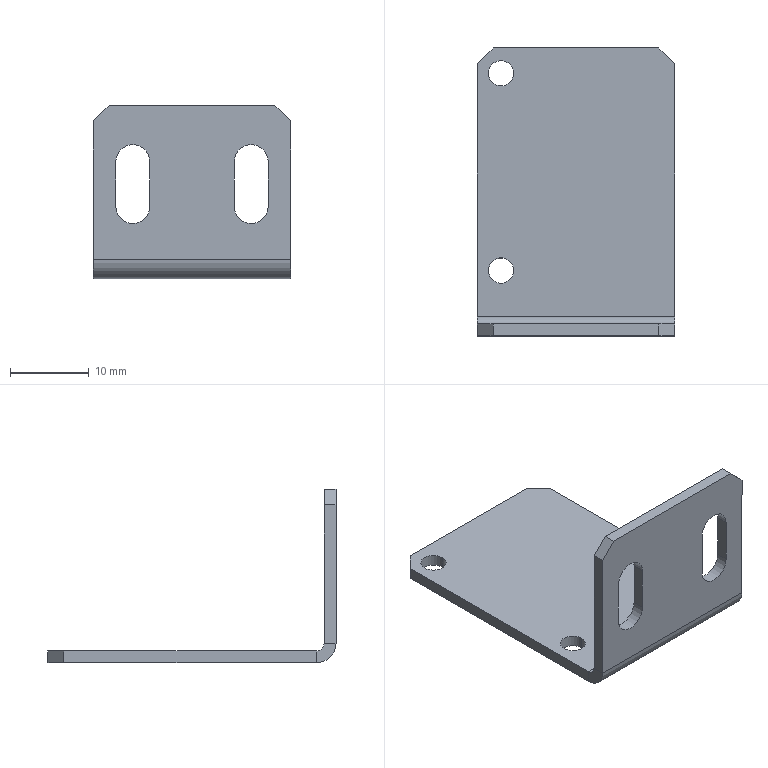Part | STEP file | FBDS-TL-005 | 1 solid | 32 faces | box 25 x 36.5 x 22 mm | volume 1956 mm3 | plane 20 | cylinder 12 | commonest cylinder face diameters 4.3 x6 3.2 x4 2 x1 5 x1
STEP:
#1=CARTESIAN_POINT('',(-7.9,-10.7,0.));
#2=VERTEX_POINT('',#1);
#3=CARTESIAN_POINT('',(-11.1,-10.7,0.));
#4=VERTEX_POINT('',#3);
#5=CARTESIAN_POINT('',(-9.5,-10.7,0.));
#6=DIRECTION('',(0.,0.,-1.));
#7=DIRECTION('',(-1.,0.,0.));
#8=AXIS2_PLACEMENT_3D('',#5,#6,#7);
#9=CIRCLE('',#8,1.6);
#10=EDGE_CURVE('',#2,#4,#9,.T.);
#11=ORIENTED_EDGE('',*,*,#10,.F.);
#12=CARTESIAN_POINT('',(-7.9,-10.7,-1.5));
#13=VERTEX_POINT('',#12);
#14=CARTESIAN_POINT('',(-7.9,-10.7,-1.5));
#15=DIRECTION('',(0.,0.,-1.));
#16=VECTOR('',#15,1000.);
#17=LINE('',#14,#16);
#18=EDGE_CURVE('',#2,#13,#17,.T.);
#19=ORIENTED_EDGE('',*,*,#18,.T.);
#20=CARTESIAN_POINT('',(-11.1,-10.7,-1.5));
#21=VERTEX_POINT('',#20);
#22=CARTESIAN_POINT('',(-9.5,-10.7,-1.5));
#23=DIRECTION('',(0.,0.,-1.));
#24=DIRECTION('',(-1.,0.,0.));
#25=AXIS2_PLACEMENT_3D('',#22,#23,#24);
#26=CIRCLE('',#25,1.6);
#27=EDGE_CURVE('',#13,#21,#26,.T.);
#28=ORIENTED_EDGE('',*,*,#27,.T.);
#29=CARTESIAN_POINT('',(-11.1,-10.7,-1.5));
#30=DIRECTION('',(0.,0.,-1.));
#31=VECTOR('',#30,1000.);
#32=LINE('',#29,#31);
#33=EDGE_CURVE('',#4,#21,#32,.T.);
#34=ORIENTED_EDGE('',*,*,#33,.F.);
#35=EDGE_LOOP('',(#11,#19,#28,#34));
#36=FACE_OUTER_BOUND('',#35,.T.);
#37=CARTESIAN_POINT('',(-9.5,-10.7,-1.5));
#38=DIRECTION('',(0.,0.,-1.));
#39=DIRECTION('',(-1.,0.,0.));
#40=AXIS2_PLACEMENT_3D('',#37,#38,#39);
#41=CYLINDRICAL_SURFACE('',#40,1.6);
#42=ADVANCED_FACE('',(#36),#41,.F.);
#43=CARTESIAN_POINT('',(-7.9,14.3,0.));
#44=VERTEX_POINT('',#43);
#45=CARTESIAN_POINT('',(-11.1,14.3,0.));
#46=VERTEX_POINT('',#45);
#47=CARTESIAN_POINT('',(-9.5,14.3,0.));
#48=DIRECTION('',(0.,0.,-1.));
#49=DIRECTION('',(-1.,0.,0.));
#50=AXIS2_PLACEMENT_3D('',#47,#48,#49);
#51=CIRCLE('',#50,1.6);
#52=EDGE_CURVE('',#44,#46,#51,.T.);
#53=ORIENTED_EDGE('',*,*,#52,.F.);
#54=CARTESIAN_POINT('',(-7.9,14.3,-1.5));
#55=VERTEX_POINT('',#54);
#56=CARTESIAN_POINT('',(-7.9,14.3,-1.5));
#57=DIRECTION('',(0.,0.,-1.));
#58=VECTOR('',#57,1000.);
#59=LINE('',#56,#58);
#60=EDGE_CURVE('',#44,#55,#59,.T.);
#61=ORIENTED_EDGE('',*,*,#60,.T.);
#62=CARTESIAN_POINT('',(-11.1,14.3,-1.5));
#63=VERTEX_POINT('',#62);
#64=CARTESIAN_POINT('',(-9.5,14.3,-1.5));
#65=DIRECTION('',(0.,0.,-1.));
#66=DIRECTION('',(-1.,0.,0.));
#67=AXIS2_PLACEMENT_3D('',#64,#65,#66);
#68=CIRCLE('',#67,1.6);
#69=EDGE_CURVE('',#55,#63,#68,.T.);
#70=ORIENTED_EDGE('',*,*,#69,.T.);
#71=CARTESIAN_POINT('',(-11.1,14.3,-1.5));
#72=DIRECTION('',(0.,0.,-1.));
#73=VECTOR('',#72,1000.);
#74=LINE('',#71,#73);
#75=EDGE_CURVE('',#46,#63,#74,.T.);
#76=ORIENTED_EDGE('',*,*,#75,.F.);
#77=EDGE_LOOP('',(#53,#61,#70,#76));
#78=FACE_OUTER_BOUND('',#77,.T.);
#79=CARTESIAN_POINT('',(-9.5,14.3,-1.5));
#80=DIRECTION('',(0.,0.,-1.));
#81=DIRECTION('',(-1.,0.,0.));
#82=AXIS2_PLACEMENT_3D('',#79,#80,#81);
#83=CYLINDRICAL_SURFACE('',#82,1.6);
#84=ADVANCED_FACE('',(#78),#83,.F.);
#85=CARTESIAN_POINT('',(-7.5,-19.,15.5));
#86=VERTEX_POINT('',#85);
#87=CARTESIAN_POINT('',(-5.35,-19.,13.35));
#88=VERTEX_POINT('',#87);
#89=CARTESIAN_POINT('',(-7.5,-19.,13.35));
#90=DIRECTION('',(0.,1.,0.));
#91=DIRECTION('',(0.,0.,1.));
#92=AXIS2_PLACEMENT_3D('',#89,#90,#91);
#93=CIRCLE('',#92,2.15);
#94=EDGE_CURVE('',#86,#88,#93,.T.);
#95=ORIENTED_EDGE('',*,*,#94,.F.);
#96=CARTESIAN_POINT('',(-7.5,-17.5,15.5));
#97=VERTEX_POINT('',#96);
#98=CARTESIAN_POINT('',(-7.5,-17.5,15.5));
#99=DIRECTION('',(0.,1.,0.));
#100=VECTOR('',#99,1000.);
#101=LINE('',#98,#100);
#102=EDGE_CURVE('',#86,#97,#101,.T.);
#103=ORIENTED_EDGE('',*,*,#102,.T.);
#104=CARTESIAN_POINT('',(-5.35,-17.5,13.35));
#105=VERTEX_POINT('',#104);
#106=CARTESIAN_POINT('',(-7.5,-17.5,13.35));
#107=DIRECTION('',(0.,1.,0.));
#108=DIRECTION('',(0.,0.,1.));
#109=AXIS2_PLACEMENT_3D('',#106,#107,#108);
#110=CIRCLE('',#109,2.15);
#111=EDGE_CURVE('',#97,#105,#110,.T.);
#112=ORIENTED_EDGE('',*,*,#111,.T.);
#113=CARTESIAN_POINT('',(-5.35,-39.9,13.35));
#114=DIRECTION('',(0.,-1.,0.));
#115=VECTOR('',#114,1000.);
#116=LINE('',#113,#115);
#117=EDGE_CURVE('',#105,#88,#116,.T.);
#118=ORIENTED_EDGE('',*,*,#117,.T.);
#119=EDGE_LOOP('',(#95,#103,#112,#118));
#120=FACE_OUTER_BOUND('',#119,.T.);
#121=CARTESIAN_POINT('',(-7.5,-17.5,13.35));
#122=DIRECTION('',(0.,1.,0.));
#123=DIRECTION('',(0.,0.,1.));
#124=AXIS2_PLACEMENT_3D('',#121,#122,#123);
#125=CYLINDRICAL_SURFACE('',#124,2.15);
#126=ADVANCED_FACE('',(#120),#125,.F.);
#127=CARTESIAN_POINT('',(7.5,-19.,15.5));
#128=VERTEX_POINT('',#127);
#129=CARTESIAN_POINT('',(9.65,-19.,13.35));
#130=VERTEX_POINT('',#129);
#131=CARTESIAN_POINT('',(7.5,-19.,13.35));
#132=DIRECTION('',(0.,1.,0.));
#133=DIRECTION('',(0.,0.,1.));
#134=AXIS2_PLACEMENT_3D('',#131,#132,#133);
#135=CIRCLE('',#134,2.15);
#136=EDGE_CURVE('',#128,#130,#135,.T.);
#137=ORIENTED_EDGE('',*,*,#136,.F.);
#138=CARTESIAN_POINT('',(7.5,-17.5,15.5));
#139=VERTEX_POINT('',#138);
#140=CARTESIAN_POINT('',(7.5,-17.5,15.5));
#141=DIRECTION('',(0.,1.,0.));
#142=VECTOR('',#141,1000.);
#143=LINE('',#140,#142);
#144=EDGE_CURVE('',#128,#139,#143,.T.);
#145=ORIENTED_EDGE('',*,*,#144,.T.);
#146=CARTESIAN_POINT('',(9.65,-17.5,13.35));
#147=VERTEX_POINT('',#146);
#148=CARTESIAN_POINT('',(7.5,-17.5,13.35));
#149=DIRECTION('',(0.,1.,0.));
#150=DIRECTION('',(0.,0.,1.));
#151=AXIS2_PLACEMENT_3D('',#148,#149,#150);
#152=CIRCLE('',#151,2.15);
#153=EDGE_CURVE('',#139,#147,#152,.T.);
#154=ORIENTED_EDGE('',*,*,#153,.T.);
#155=CARTESIAN_POINT('',(9.65,-39.9,13.35));
#156=DIRECTION('',(0.,-1.,0.));
#157=VECTOR('',#156,1000.);
#158=LINE('',#155,#157);
#159=EDGE_CURVE('',#147,#130,#158,.T.);
#160=ORIENTED_EDGE('',*,*,#159,.T.);
#161=EDGE_LOOP('',(#137,#145,#154,#160));
#162=FACE_OUTER_BOUND('',#161,.T.);
#163=CARTESIAN_POINT('',(7.5,-17.5,13.35));
#164=DIRECTION('',(0.,1.,0.));
#165=DIRECTION('',(0.,0.,1.));
#166=AXIS2_PLACEMENT_3D('',#163,#164,#165);
#167=CYLINDRICAL_SURFACE('',#166,2.15);
#168=ADVANCED_FACE('',(#162),#167,.F.);
#169=CARTESIAN_POINT('',(12.5,-16.5,-1.5));
#170=VERTEX_POINT('',#169);
#171=CARTESIAN_POINT('',(12.5,15.5,-1.5));
#172=VERTEX_POINT('',#171);
#173=CARTESIAN_POINT('',(12.5,-17.5,-1.5));
#174=DIRECTION('',(0.,1.,0.));
#175=VECTOR('',#174,1000.);
#176=LINE('',#173,#175);
#177=EDGE_CURVE('',#170,#172,#176,.T.);
#178=ORIENTED_EDGE('',*,*,#177,.T.);
#179=CARTESIAN_POINT('',(12.5,15.5,0.));
#180=VERTEX_POINT('',#179);
#181=CARTESIAN_POINT('',(12.5,15.5,-1.5));
#182=DIRECTION('',(0.,0.,1.));
#183=VECTOR('',#182,1000.);
#184=LINE('',#181,#183);
#185=EDGE_CURVE('',#172,#180,#184,.T.);
#186=ORIENTED_EDGE('',*,*,#185,.T.);
#187=CARTESIAN_POINT('',(12.5,-16.5,0.));
#188=VERTEX_POINT('',#187);
#189=CARTESIAN_POINT('',(12.5,-17.5,0.));
#190=DIRECTION('',(0.,1.,0.));
#191=VECTOR('',#190,1000.);
#192=LINE('',#189,#191);
#193=EDGE_CURVE('',#188,#180,#192,.T.);
#194=ORIENTED_EDGE('',*,*,#193,.F.);
#195=CARTESIAN_POINT('',(12.5,-16.5,0.));
#196=DIRECTION('',(0.,0.,-1.));
#197=VECTOR('',#196,1000.);
#198=LINE('',#195,#197);
#199=EDGE_CURVE('',#188,#170,#198,.T.);
#200=ORIENTED_EDGE('',*,*,#199,.T.);
#201=EDGE_LOOP('',(#178,#186,#194,#200));
#202=FACE_OUTER_BOUND('',#201,.T.);
#203=CARTESIAN_POINT('',(12.5,-17.5,-1.5));
#204=DIRECTION('',(1.,0.,0.));
#205=DIRECTION('',(0.,0.,-1.));
#206=AXIS2_PLACEMENT_3D('',#203,#204,#205);
#207=PLANE('',#206);
#208=ADVANCED_FACE('',(#202),#207,.T.);
#209=CARTESIAN_POINT('',(-9.5,-10.7,-1.5));
#210=DIRECTION('',(0.,0.,-1.));
#211=DIRECTION('',(-1.,0.,0.));
#212=AXIS2_PLACEMENT_3D('',#209,#210,#211);
#213=CIRCLE('',#212,1.6);
#214=EDGE_CURVE('',#21,#13,#213,.T.);
#215=ORIENTED_EDGE('',*,*,#214,.F.);
#216=ORIENTED_EDGE('',*,*,#27,.F.);
#217=EDGE_LOOP('',(#215,#216));
#218=FACE_BOUND('',#217,.T.);
#219=CARTESIAN_POINT('',(-9.5,14.3,-1.5));
#220=DIRECTION('',(0.,0.,-1.));
#221=DIRECTION('',(-1.,0.,0.));
#222=AXIS2_PLACEMENT_3D('',#219,#220,#221);
#223=CIRCLE('',#222,1.6);
#224=EDGE_CURVE('',#63,#55,#223,.T.);
#225=ORIENTED_EDGE('',*,*,#224,.F.);
#226=ORIENTED_EDGE('',*,*,#69,.F.);
#227=EDGE_LOOP('',(#225,#226));
#228=FACE_BOUND('',#227,.T.);
#229=CARTESIAN_POINT('',(-12.5,15.5,-1.5));
#230=VERTEX_POINT('',#229);
#231=CARTESIAN_POINT('',(-12.5,-16.5,-1.5));
#232=VERTEX_POINT('',#231);
#233=CARTESIAN_POINT('',(-12.5,-17.5,-1.5));
#234=DIRECTION('',(0.,-1.,0.));
#235=VECTOR('',#234,1000.);
#236=LINE('',#233,#235);
#237=EDGE_CURVE('',#230,#232,#236,.T.);
#238=ORIENTED_EDGE('',*,*,#237,.F.);
#239=CARTESIAN_POINT('',(-10.5,17.5,-1.5));
#240=VERTEX_POINT('',#239);
#241=CARTESIAN_POINT('',(-14.,14.,-1.5));
#242=DIRECTION('',(0.7071,0.7071,0.));
#243=VECTOR('',#242,1000.);
#244=LINE('',#241,#243);
#245=EDGE_CURVE('',#230,#240,#244,.T.);
#246=ORIENTED_EDGE('',*,*,#245,.T.);
#247=CARTESIAN_POINT('',(10.5,17.5,-1.5));
#248=VERTEX_POINT('',#247);
#249=CARTESIAN_POINT('',(-12.5,17.5,-1.5));
#250=DIRECTION('',(-1.,0.,0.));
#251=VECTOR('',#250,1000.);
#252=LINE('',#249,#251);
#253=EDGE_CURVE('',#248,#240,#252,.T.);
#254=ORIENTED_EDGE('',*,*,#253,.F.);
#255=CARTESIAN_POINT('',(14.,14.,-1.5));
#256=DIRECTION('',(0.7071,-0.7071,0.));
#257=VECTOR('',#256,1000.);
#258=LINE('',#255,#257);
#259=EDGE_CURVE('',#248,#172,#258,.T.);
#260=ORIENTED_EDGE('',*,*,#259,.T.);
#261=ORIENTED_EDGE('',*,*,#177,.F.);
#262=CARTESIAN_POINT('',(12.5,-16.5,-1.5));
#263=DIRECTION('',(-1.,0.,0.));
#264=VECTOR('',#263,1000.);
#265=LINE('',#262,#264);
#266=EDGE_CURVE('',#170,#232,#265,.T.);
#267=ORIENTED_EDGE('',*,*,#266,.T.);
#268=EDGE_LOOP('',(#238,#246,#254,#260,#261,#267));
#269=FACE_OUTER_BOUND('',#268,.T.);
#270=CARTESIAN_POINT('',(0.,0.,-1.5));
#271=DIRECTION('',(0.,0.,-1.));
#272=DIRECTION('',(-1.,0.,0.));
#273=AXIS2_PLACEMENT_3D('',#270,#271,#272);
#274=PLANE('',#273);
#275=ADVANCED_FACE('',(#218,#228,#269),#274,.T.);
#276=CARTESIAN_POINT('',(-9.5,-10.7,0.));
#277=DIRECTION('',(0.,0.,-1.));
#278=DIRECTION('',(-1.,0.,0.));
#279=AXIS2_PLACEMENT_3D('',#276,#277,#278);
#280=CIRCLE('',#279,1.6);
#281=EDGE_CURVE('',#4,#2,#280,.T.);
#282=ORIENTED_EDGE('',*,*,#281,.T.);
#283=ORIENTED_EDGE('',*,*,#10,.T.);
#284=EDGE_LOOP('',(#282,#283));
#285=FACE_BOUND('',#284,.T.);
#286=CARTESIAN_POINT('',(-9.5,14.3,0.));
#287=DIRECTION('',(0.,0.,-1.));
#288=DIRECTION('',(-1.,0.,0.));
#289=AXIS2_PLACEMENT_3D('',#286,#287,#288);
#290=CIRCLE('',#289,1.6);
#291=EDGE_CURVE('',#46,#44,#290,.T.);
#292=ORIENTED_EDGE('',*,*,#291,.T.);
#293=ORIENTED_EDGE('',*,*,#52,.T.);
#294=EDGE_LOOP('',(#292,#293));
#295=FACE_BOUND('',#294,.T.);
#296=CARTESIAN_POINT('',(10.5,17.5,0.));
#297=VERTEX_POINT('',#296);
#298=CARTESIAN_POINT('',(-10.5,17.5,0.));
#299=VERTEX_POINT('',#298);
#300=CARTESIAN_POINT('',(-12.5,17.5,0.));
#301=DIRECTION('',(-1.,0.,0.));
#302=VECTOR('',#301,1000.);
#303=LINE('',#300,#302);
#304=EDGE_CURVE('',#297,#299,#303,.T.);
#305=ORIENTED_EDGE('',*,*,#304,.T.);
#306=CARTESIAN_POINT('',(-12.5,15.5,0.));
#307=VERTEX_POINT('',#306);
#308=CARTESIAN_POINT('',(-10.5,17.5,0.));
#309=DIRECTION('',(-0.7071,-0.7071,0.));
#310=VECTOR('',#309,1000.);
#311=LINE('',#308,#310);
#312=EDGE_CURVE('',#299,#307,#311,.T.);
#313=ORIENTED_EDGE('',*,*,#312,.T.);
#314=CARTESIAN_POINT('',(-12.5,-16.5,0.));
#315=VERTEX_POINT('',#314);
#316=CARTESIAN_POINT('',(-12.5,-17.5,0.));
#317=DIRECTION('',(0.,-1.,0.));
#318=VECTOR('',#317,1000.);
#319=LINE('',#316,#318);
#320=EDGE_CURVE('',#307,#315,#319,.T.);
#321=ORIENTED_EDGE('',*,*,#320,.T.);
#322=CARTESIAN_POINT('',(12.5,-16.5,0.));
#323=DIRECTION('',(-1.,0.,0.));
#324=VECTOR('',#323,1000.);
#325=LINE('',#322,#324);
#326=EDGE_CURVE('',#188,#315,#325,.T.);
#327=ORIENTED_EDGE('',*,*,#326,.F.);
#328=ORIENTED_EDGE('',*,*,#193,.T.);
#329=CARTESIAN_POINT('',(12.5,15.5,0.));
#330=DIRECTION('',(-0.7071,0.7071,0.));
#331=VECTOR('',#330,1000.);
#332=LINE('',#329,#331);
#333=EDGE_CURVE('',#180,#297,#332,.T.);
#334=ORIENTED_EDGE('',*,*,#333,.T.);
#335=EDGE_LOOP('',(#305,#313,#321,#327,#328,#334));
#336=FACE_OUTER_BOUND('',#335,.T.);
#337=CARTESIAN_POINT('',(0.,0.,0.));
#338=DIRECTION('',(0.,0.,-1.));
#339=DIRECTION('',(-1.,0.,0.));
#340=AXIS2_PLACEMENT_3D('',#337,#338,#339);
#341=PLANE('',#340);
#342=ADVANCED_FACE('',(#285,#295,#336),#341,.F.);
#343=ORIENTED_EDGE('',*,*,#320,.F.);
#344=CARTESIAN_POINT('',(-12.5,15.5,-1.5));
#345=DIRECTION('',(0.,0.,-1.));
#346=VECTOR('',#345,1000.);
#347=LINE('',#344,#346);
#348=EDGE_CURVE('',#307,#230,#347,.T.);
#349=ORIENTED_EDGE('',*,*,#348,.T.);
#350=ORIENTED_EDGE('',*,*,#237,.T.);
#351=CARTESIAN_POINT('',(-12.5,-16.5,0.));
#352=DIRECTION('',(0.,0.,-1.));
#353=VECTOR('',#352,1000.);
#354=LINE('',#351,#353);
#355=EDGE_CURVE('',#315,#232,#354,.T.);
#356=ORIENTED_EDGE('',*,*,#355,.F.);
#357=EDGE_LOOP('',(#343,#349,#350,#356));
#358=FACE_OUTER_BOUND('',#357,.T.);
#359=CARTESIAN_POINT('',(-12.5,-17.5,-1.5));
#360=DIRECTION('',(-1.,0.,0.));
#361=DIRECTION('',(0.,0.,1.));
#362=AXIS2_PLACEMENT_3D('',#359,#360,#361);
#363=PLANE('',#362);
#364=ADVANCED_FACE('',(#358),#363,.T.);
#365=ORIENTED_EDGE('',*,*,#253,.T.);
#366=CARTESIAN_POINT('',(-10.5,17.5,-1.5));
#367=DIRECTION('',(0.,0.,1.));
#368=VECTOR('',#367,1000.);
#369=LINE('',#366,#368);
#370=EDGE_CURVE('',#240,#299,#369,.T.);
#371=ORIENTED_EDGE('',*,*,#370,.T.);
#372=ORIENTED_EDGE('',*,*,#304,.F.);
#373=CARTESIAN_POINT('',(10.5,17.5,-1.5));
#374=DIRECTION('',(0.,0.,-1.));
#375=VECTOR('',#374,1000.);
#376=LINE('',#373,#375);
#377=EDGE_CURVE('',#297,#248,#376,.T.);
#378=ORIENTED_EDGE('',*,*,#377,.T.);
#379=EDGE_LOOP('',(#365,#371,#372,#378));
#380=FACE_OUTER_BOUND('',#379,.T.);
#381=CARTESIAN_POINT('',(-12.5,17.5,-1.5));
#382=DIRECTION('',(0.,1.,0.));
#383=DIRECTION('',(0.,0.,1.));
#384=AXIS2_PLACEMENT_3D('',#381,#382,#383);
#385=PLANE('',#384);
#386=ADVANCED_FACE('',(#380),#385,.T.);
#387=CARTESIAN_POINT('',(-12.5,-17.5,1.));
#388=VERTEX_POINT('',#387);
#389=CARTESIAN_POINT('',(-12.5,-19.,1.));
#390=VERTEX_POINT('',#389);
#391=CARTESIAN_POINT('',(-12.5,-17.5,1.));
#392=DIRECTION('',(0.,-1.,0.));
#393=VECTOR('',#392,1000.);
#394=LINE('',#391,#393);
#395=EDGE_CURVE('',#388,#390,#394,.T.);
#396=ORIENTED_EDGE('',*,*,#395,.F.);
#397=CARTESIAN_POINT('',(-12.5,-16.5,1.));
#398=DIRECTION('',(-1.,0.,0.));
#399=DIRECTION('',(0.,0.,-1.));
#400=AXIS2_PLACEMENT_3D('',#397,#398,#399);
#401=CIRCLE('',#400,1.);
#402=EDGE_CURVE('',#315,#388,#401,.T.);
#403=ORIENTED_EDGE('',*,*,#402,.F.);
#404=ORIENTED_EDGE('',*,*,#355,.T.);
#405=CARTESIAN_POINT('',(-12.5,-16.5,1.));
#406=DIRECTION('',(-1.,0.,0.));
#407=DIRECTION('',(0.,0.,-1.));
#408=AXIS2_PLACEMENT_3D('',#405,#406,#407);
#409=CIRCLE('',#408,2.5);
#410=EDGE_CURVE('',#232,#390,#409,.T.);
#411=ORIENTED_EDGE('',*,*,#410,.T.);
#412=EDGE_LOOP('',(#396,#403,#404,#411));
#413=FACE_OUTER_BOUND('',#412,.T.);
#414=CARTESIAN_POINT('',(-12.5,-16.5,1.));
#415=DIRECTION('',(-1.,0.,0.));
#416=DIRECTION('',(0.,0.,1.));
#417=AXIS2_PLACEMENT_3D('',#414,#415,#416);
#418=PLANE('',#417);
#419=ADVANCED_FACE('',(#413),#418,.T.);
#420=CARTESIAN_POINT('',(12.5,-17.5,1.));
#421=VERTEX_POINT('',#420);
#422=CARTESIAN_POINT('',(12.5,-16.5,1.));
#423=DIRECTION('',(1.,0.,0.));
#424=DIRECTION('',(0.,0.,-1.));
#425=AXIS2_PLACEMENT_3D('',#422,#423,#424);
#426=CIRCLE('',#425,1.);
#427=EDGE_CURVE('',#421,#188,#426,.T.);
#428=ORIENTED_EDGE('',*,*,#427,.F.);
#429=CARTESIAN_POINT('',(12.5,-19.,1.));
#430=VERTEX_POINT('',#429);
#431=CARTESIAN_POINT('',(12.5,-17.5,1.));
#432=DIRECTION('',(0.,-1.,0.));
#433=VECTOR('',#432,1000.);
#434=LINE('',#431,#433);
#435=EDGE_CURVE('',#421,#430,#434,.T.);
#436=ORIENTED_EDGE('',*,*,#435,.T.);
#437=CARTESIAN_POINT('',(12.5,-16.5,1.));
#438=DIRECTION('',(1.,0.,0.));
#439=DIRECTION('',(0.,0.,-1.));
#440=AXIS2_PLACEMENT_3D('',#437,#438,#439);
#441=CIRCLE('',#440,2.5);
#442=EDGE_CURVE('',#430,#170,#441,.T.);
#443=ORIENTED_EDGE('',*,*,#442,.T.);
#444=ORIENTED_EDGE('',*,*,#199,.F.);
#445=EDGE_LOOP('',(#428,#436,#443,#444));
#446=FACE_OUTER_BOUND('',#445,.T.);
#447=CARTESIAN_POINT('',(12.5,-16.5,1.));
#448=DIRECTION('',(-1.,0.,0.));
#449=DIRECTION('',(0.,0.,1.));
#450=AXIS2_PLACEMENT_3D('',#447,#448,#449);
#451=PLANE('',#450);
#452=ADVANCED_FACE('',(#446),#451,.F.);
#453=ORIENTED_EDGE('',*,*,#266,.F.);
#454=ORIENTED_EDGE('',*,*,#442,.F.);
#455=CARTESIAN_POINT('',(0.,-19.,1.));
#456=DIRECTION('',(-1.,0.,0.));
#457=VECTOR('',#456,1000.);
#458=LINE('',#455,#457);
#459=EDGE_CURVE('',#430,#390,#458,.T.);
#460=ORIENTED_EDGE('',*,*,#459,.T.);
#461=ORIENTED_EDGE('',*,*,#410,.F.);
#462=EDGE_LOOP('',(#453,#454,#460,#461));
#463=FACE_OUTER_BOUND('',#462,.T.);
#464=CARTESIAN_POINT('',(12.5,-16.5,1.));
#465=DIRECTION('',(1.,0.,0.));
#466=DIRECTION('',(0.,-1.,0.));
#467=AXIS2_PLACEMENT_3D('',#464,#465,#466);
#468=CYLINDRICAL_SURFACE('',#467,2.5);
#469=ADVANCED_FACE('',(#463),#468,.T.);
#470=ORIENTED_EDGE('',*,*,#326,.T.);
#471=ORIENTED_EDGE('',*,*,#402,.T.);
#472=CARTESIAN_POINT('',(-12.5,-17.5,1.));
#473=DIRECTION('',(1.,0.,0.));
#474=VECTOR('',#473,1000.);
#475=LINE('',#472,#474);
#476=EDGE_CURVE('',#388,#421,#475,.T.);
#477=ORIENTED_EDGE('',*,*,#476,.T.);
#478=ORIENTED_EDGE('',*,*,#427,.T.);
#479=EDGE_LOOP('',(#470,#471,#477,#478));
#480=FACE_OUTER_BOUND('',#479,.T.);
#481=CARTESIAN_POINT('',(12.5,-16.5,1.));
#482=DIRECTION('',(1.,0.,0.));
#483=DIRECTION('',(0.,-1.,0.));
#484=AXIS2_PLACEMENT_3D('',#481,#482,#483);
#485=CYLINDRICAL_SURFACE('',#484,1.);
#486=ADVANCED_FACE('',(#480),#485,.F.);
#487=CARTESIAN_POINT('',(-12.5,-19.,18.5));
#488=VERTEX_POINT('',#487);
#489=CARTESIAN_POINT('',(-12.5,-19.,0.));
#490=DIRECTION('',(0.,0.,-1.));
#491=VECTOR('',#490,1000.);
#492=LINE('',#489,#491);
#493=EDGE_CURVE('',#488,#390,#492,.T.);
#494=ORIENTED_EDGE('',*,*,#493,.F.);
#495=CARTESIAN_POINT('',(-12.5,-17.5,18.5));
#496=VERTEX_POINT('',#495);
#497=CARTESIAN_POINT('',(-12.5,-19.,18.5));
#498=DIRECTION('',(0.,1.,0.));
#499=VECTOR('',#498,1000.);
#500=LINE('',#497,#499);
#501=EDGE_CURVE('',#488,#496,#500,.T.);
#502=ORIENTED_EDGE('',*,*,#501,.T.);
#503=CARTESIAN_POINT('',(-12.5,-17.5,0.));
#504=DIRECTION('',(0.,0.,-1.));
#505=VECTOR('',#504,1000.);
#506=LINE('',#503,#505);
#507=EDGE_CURVE('',#496,#388,#506,.T.);
#508=ORIENTED_EDGE('',*,*,#507,.T.);
#509=ORIENTED_EDGE('',*,*,#395,.T.);
#510=EDGE_LOOP('',(#494,#502,#508,#509));
#511=FACE_OUTER_BOUND('',#510,.T.);
#512=CARTESIAN_POINT('',(-12.5,-19.,0.));
#513=DIRECTION('',(1.,0.,0.));
#514=DIRECTION('',(0.,0.,-1.));
#515=AXIS2_PLACEMENT_3D('',#512,#513,#514);
#516=PLANE('',#515);
#517=ADVANCED_FACE('',(#511),#516,.F.);
#518=CARTESIAN_POINT('',(12.5,-17.5,18.5));
#519=VERTEX_POINT('',#518);
#520=CARTESIAN_POINT('',(12.5,-17.5,20.5));
#521=DIRECTION('',(0.,0.,1.));
#522=VECTOR('',#521,1000.);
#523=LINE('',#520,#522);
#524=EDGE_CURVE('',#421,#519,#523,.T.);
#525=ORIENTED_EDGE('',*,*,#524,.T.);
#526=CARTESIAN_POINT('',(12.5,-19.,18.5));
#527=VERTEX_POINT('',#526);
#528=CARTESIAN_POINT('',(12.5,-19.,18.5));
#529=DIRECTION('',(0.,-1.,0.));
#530=VECTOR('',#529,1000.);
#531=LINE('',#528,#530);
#532=EDGE_CURVE('',#519,#527,#531,.T.);
#533=ORIENTED_EDGE('',*,*,#532,.T.);
#534=CARTESIAN_POINT('',(12.5,-19.,20.5));
#535=DIRECTION('',(0.,0.,1.));
#536=VECTOR('',#535,1000.);
#537=LINE('',#534,#536);
#538=EDGE_CURVE('',#430,#527,#537,.T.);
#539=ORIENTED_EDGE('',*,*,#538,.F.);
#540=ORIENTED_EDGE('',*,*,#435,.F.);
#541=EDGE_LOOP('',(#525,#533,#539,#540));
#542=FACE_OUTER_BOUND('',#541,.T.);
#543=CARTESIAN_POINT('',(12.5,-19.,20.5));
#544=DIRECTION('',(-1.,0.,0.));
#545=DIRECTION('',(0.,0.,1.));
#546=AXIS2_PLACEMENT_3D('',#543,#544,#545);
#547=PLANE('',#546);
#548=ADVANCED_FACE('',(#542),#547,.F.);
#549=CARTESIAN_POINT('',(-9.65,-19.,13.35));
#550=VERTEX_POINT('',#549);
#551=CARTESIAN_POINT('',(-7.5,-19.,13.35));
#552=DIRECTION('',(0.,1.,0.));
#553=DIRECTION('',(0.,0.,1.));
#554=AXIS2_PLACEMENT_3D('',#551,#552,#553);
#555=CIRCLE('',#554,2.15);
#556=EDGE_CURVE('',#550,#86,#555,.T.);
#557=ORIENTED_EDGE('',*,*,#556,.T.);
#558=ORIENTED_EDGE('',*,*,#94,.T.);
#559=CARTESIAN_POINT('',(-5.35,-19.,7.65));
#560=VERTEX_POINT('',#559);
#561=CARTESIAN_POINT('',(-5.35,-19.,0.));
#562=DIRECTION('',(0.,0.,-1.));
#563=VECTOR('',#562,1000.);
#564=LINE('',#561,#563);
#565=EDGE_CURVE('',#88,#560,#564,.T.);
#566=ORIENTED_EDGE('',*,*,#565,.T.);
#567=CARTESIAN_POINT('',(-9.65,-19.,7.65));
#568=VERTEX_POINT('',#567);
#569=CARTESIAN_POINT('',(-7.5,-19.,7.65));
#570=DIRECTION('',(0.,1.,0.));
#571=DIRECTION('',(0.,0.,1.));
#572=AXIS2_PLACEMENT_3D('',#569,#570,#571);
#573=CIRCLE('',#572,2.15);
#574=EDGE_CURVE('',#560,#568,#573,.T.);
#575=ORIENTED_EDGE('',*,*,#574,.T.);
#576=CARTESIAN_POINT('',(-9.65,-19.,0.));
#577=DIRECTION('',(0.,0.,1.));
#578=VECTOR('',#577,1000.);
#579=LINE('',#576,#578);
#580=EDGE_CURVE('',#568,#550,#579,.T.);
#581=ORIENTED_EDGE('',*,*,#580,.T.);
#582=EDGE_LOOP('',(#557,#558,#566,#575,#581));
#583=FACE_BOUND('',#582,.T.);
#584=CARTESIAN_POINT('',(5.35,-19.,7.65));
#585=VERTEX_POINT('',#584);
#586=CARTESIAN_POINT('',(5.35,-19.,13.35));
#587=VERTEX_POINT('',#586);
#588=CARTESIAN_POINT('',(5.35,-19.,0.));
#589=DIRECTION('',(0.,0.,1.));
#590=VECTOR('',#589,1000.);
#591=LINE('',#588,#590);
#592=EDGE_CURVE('',#585,#587,#591,.T.);
#593=ORIENTED_EDGE('',*,*,#592,.T.);
#594=CARTESIAN_POINT('',(7.5,-19.,13.35));
#595=DIRECTION('',(0.,1.,0.));
#596=DIRECTION('',(0.,0.,1.));
#597=AXIS2_PLACEMENT_3D('',#594,#595,#596);
#598=CIRCLE('',#597,2.15);
#599=EDGE_CURVE('',#587,#128,#598,.T.);
#600=ORIENTED_EDGE('',*,*,#599,.T.);
#601=ORIENTED_EDGE('',*,*,#136,.T.);
#602=CARTESIAN_POINT('',(9.65,-19.,7.65));
#603=VERTEX_POINT('',#602);
#604=CARTESIAN_POINT('',(9.65,-19.,0.));
#605=DIRECTION('',(0.,0.,-1.));
#606=VECTOR('',#605,1000.);
#607=LINE('',#604,#606);
#608=EDGE_CURVE('',#130,#603,#607,.T.);
#609=ORIENTED_EDGE('',*,*,#608,.T.);
#610=CARTESIAN_POINT('',(7.5,-19.,7.65));
#611=DIRECTION('',(0.,1.,0.));
#612=DIRECTION('',(0.,0.,1.));
#613=AXIS2_PLACEMENT_3D('',#610,#611,#612);
#614=CIRCLE('',#613,2.15);
#615=EDGE_CURVE('',#603,#585,#614,.T.);
#616=ORIENTED_EDGE('',*,*,#615,.T.);
#617=EDGE_LOOP('',(#593,#600,#601,#609,#616));
#618=FACE_BOUND('',#617,.T.);
#619=CARTESIAN_POINT('',(10.5,-19.,20.5));
#620=VERTEX_POINT('',#619);
#621=CARTESIAN_POINT('',(-10.5,-19.,20.5));
#622=VERTEX_POINT('',#621);
#623=CARTESIAN_POINT('',(-12.5,-19.,20.5));
#624=DIRECTION('',(-1.,0.,0.));
#625=VECTOR('',#624,1000.);
#626=LINE('',#623,#625);
#627=EDGE_CURVE('',#620,#622,#626,.T.);
#628=ORIENTED_EDGE('',*,*,#627,.T.);
#629=CARTESIAN_POINT('',(-12.5,-19.,18.5));
#630=DIRECTION('',(-0.7071,0.,-0.7071));
#631=VECTOR('',#630,1000.);
#632=LINE('',#629,#631);
#633=EDGE_CURVE('',#622,#488,#632,.T.);
#634=ORIENTED_EDGE('',*,*,#633,.T.);
#635=ORIENTED_EDGE('',*,*,#493,.T.);
#636=ORIENTED_EDGE('',*,*,#459,.F.);
#637=ORIENTED_EDGE('',*,*,#538,.T.);
#638=CARTESIAN_POINT('',(10.5,-19.,20.5));
#639=DIRECTION('',(-0.7071,0.,0.7071));
#640=VECTOR('',#639,1000.);
#641=LINE('',#638,#640);
#642=EDGE_CURVE('',#527,#620,#641,.T.);
#643=ORIENTED_EDGE('',*,*,#642,.T.);
#644=EDGE_LOOP('',(#628,#634,#635,#636,#637,#643));
#645=FACE_OUTER_BOUND('',#644,.T.);
#646=CARTESIAN_POINT('',(0.,-19.,0.));
#647=DIRECTION('',(0.,1.,0.));
#648=DIRECTION('',(0.,0.,1.));
#649=AXIS2_PLACEMENT_3D('',#646,#647,#648);
#650=PLANE('',#649);
#651=ADVANCED_FACE('',(#583,#618,#645),#650,.F.);
#652=CARTESIAN_POINT('',(-5.35,-17.5,7.65));
#653=VERTEX_POINT('',#652);
#654=CARTESIAN_POINT('',(-9.65,-17.5,7.65));
#655=VERTEX_POINT('',#654);
#656=CARTESIAN_POINT('',(-7.5,-17.5,7.65));
#657=DIRECTION('',(0.,1.,0.));
#658=DIRECTION('',(0.,0.,1.));
#659=AXIS2_PLACEMENT_3D('',#656,#657,#658);
#660=CIRCLE('',#659,2.15);
#661=EDGE_CURVE('',#653,#655,#660,.T.);
#662=ORIENTED_EDGE('',*,*,#661,.F.);
#663=CARTESIAN_POINT('',(-5.35,-17.5,13.35));
#664=DIRECTION('',(0.,0.,-1.));
#665=VECTOR('',#664,1000.);
#666=LINE('',#663,#665);
#667=EDGE_CURVE('',#105,#653,#666,.T.);
#668=ORIENTED_EDGE('',*,*,#667,.F.);
#669=ORIENTED_EDGE('',*,*,#111,.F.);
#670=CARTESIAN_POINT('',(-9.65,-17.5,13.35));
#671=VERTEX_POINT('',#670);
#672=CARTESIAN_POINT('',(-7.5,-17.5,13.35));
#673=DIRECTION('',(0.,1.,0.));
#674=DIRECTION('',(0.,0.,1.));
#675=AXIS2_PLACEMENT_3D('',#672,#673,#674);
#676=CIRCLE('',#675,2.15);
#677=EDGE_CURVE('',#671,#97,#676,.T.);
#678=ORIENTED_EDGE('',*,*,#677,.F.);
#679=CARTESIAN_POINT('',(-9.65,-17.5,13.35));
#680=DIRECTION('',(0.,0.,-1.));
#681=VECTOR('',#680,1000.);
#682=LINE('',#679,#681);
#683=EDGE_CURVE('',#671,#655,#682,.T.);
#684=ORIENTED_EDGE('',*,*,#683,.T.);
#685=EDGE_LOOP('',(#662,#668,#669,#678,#684));
#686=FACE_BOUND('',#685,.T.);
#687=CARTESIAN_POINT('',(9.65,-17.5,7.65));
#688=VERTEX_POINT('',#687);
#689=CARTESIAN_POINT('',(5.35,-17.5,7.65));
#690=VERTEX_POINT('',#689);
#691=CARTESIAN_POINT('',(7.5,-17.5,7.65));
#692=DIRECTION('',(0.,1.,0.));
#693=DIRECTION('',(0.,0.,1.));
#694=AXIS2_PLACEMENT_3D('',#691,#692,#693);
#695=CIRCLE('',#694,2.15);
#696=EDGE_CURVE('',#688,#690,#695,.T.);
#697=ORIENTED_EDGE('',*,*,#696,.F.);
#698=CARTESIAN_POINT('',(9.65,-17.5,13.35));
#699=DIRECTION('',(0.,0.,-1.));
#700=VECTOR('',#699,1000.);
#701=LINE('',#698,#700);
#702=EDGE_CURVE('',#147,#688,#701,.T.);
#703=ORIENTED_EDGE('',*,*,#702,.F.);
#704=ORIENTED_EDGE('',*,*,#153,.F.);
#705=CARTESIAN_POINT('',(5.35,-17.5,13.35));
#706=VERTEX_POINT('',#705);
#707=CARTESIAN_POINT('',(7.5,-17.5,13.35));
#708=DIRECTION('',(0.,1.,0.));
#709=DIRECTION('',(0.,0.,1.));
#710=AXIS2_PLACEMENT_3D('',#707,#708,#709);
#711=CIRCLE('',#710,2.15);
#712=EDGE_CURVE('',#706,#139,#711,.T.);
#713=ORIENTED_EDGE('',*,*,#712,.F.);
#714=CARTESIAN_POINT('',(5.35,-17.5,13.35));
#715=DIRECTION('',(0.,0.,-1.));
#716=VECTOR('',#715,1000.);
#717=LINE('',#714,#716);
#718=EDGE_CURVE('',#706,#690,#717,.T.);
#719=ORIENTED_EDGE('',*,*,#718,.T.);
#720=EDGE_LOOP('',(#697,#703,#704,#713,#719));
#721=FACE_BOUND('',#720,.T.);
#722=ORIENTED_EDGE('',*,*,#507,.F.);
#723=CARTESIAN_POINT('',(-10.5,-17.5,20.5));
#724=VERTEX_POINT('',#723);
#725=CARTESIAN_POINT('',(-15.5,-17.5,15.5));
#726=DIRECTION('',(0.7071,0.,0.7071));
#727=VECTOR('',#726,1000.);
#728=LINE('',#725,#727);
#729=EDGE_CURVE('',#496,#724,#728,.T.);
#730=ORIENTED_EDGE('',*,*,#729,.T.);
#731=CARTESIAN_POINT('',(10.5,-17.5,20.5));
#732=VERTEX_POINT('',#731);
#733=CARTESIAN_POINT('',(-12.5,-17.5,20.5));
#734=DIRECTION('',(-1.,0.,0.));
#735=VECTOR('',#734,1000.);
#736=LINE('',#733,#735);
#737=EDGE_CURVE('',#732,#724,#736,.T.);
#738=ORIENTED_EDGE('',*,*,#737,.F.);
#739=CARTESIAN_POINT('',(15.5,-17.5,15.5));
#740=DIRECTION('',(0.7071,0.,-0.7071));
#741=VECTOR('',#740,1000.);
#742=LINE('',#739,#741);
#743=EDGE_CURVE('',#732,#519,#742,.T.);
#744=ORIENTED_EDGE('',*,*,#743,.T.);
#745=ORIENTED_EDGE('',*,*,#524,.F.);
#746=ORIENTED_EDGE('',*,*,#476,.F.);
#747=EDGE_LOOP('',(#722,#730,#738,#744,#745,#746));
#748=FACE_OUTER_BOUND('',#747,.T.);
#749=CARTESIAN_POINT('',(0.,-17.5,0.));
#750=DIRECTION('',(0.,1.,0.));
#751=DIRECTION('',(0.,0.,1.));
#752=AXIS2_PLACEMENT_3D('',#749,#750,#751);
#753=PLANE('',#752);
#754=ADVANCED_FACE('',(#686,#721,#748),#753,.T.);
#755=ORIENTED_EDGE('',*,*,#737,.T.);
#756=CARTESIAN_POINT('',(-10.5,-19.,20.5));
#757=DIRECTION('',(0.,-1.,0.));
#758=VECTOR('',#757,1000.);
#759=LINE('',#756,#758);
#760=EDGE_CURVE('',#724,#622,#759,.T.);
#761=ORIENTED_EDGE('',*,*,#760,.T.);
#762=ORIENTED_EDGE('',*,*,#627,.F.);
#763=CARTESIAN_POINT('',(10.5,-19.,20.5));
#764=DIRECTION('',(0.,1.,0.));
#765=VECTOR('',#764,1000.);
#766=LINE('',#763,#765);
#767=EDGE_CURVE('',#620,#732,#766,.T.);
#768=ORIENTED_EDGE('',*,*,#767,.T.);
#769=EDGE_LOOP('',(#755,#761,#762,#768));
#770=FACE_OUTER_BOUND('',#769,.T.);
#771=CARTESIAN_POINT('',(-12.5,-19.,20.5));
#772=DIRECTION('',(0.,0.,-1.));
#773=DIRECTION('',(0.,1.,0.));
#774=AXIS2_PLACEMENT_3D('',#771,#772,#773);
#775=PLANE('',#774);
#776=ADVANCED_FACE('',(#770),#775,.F.);
#777=CARTESIAN_POINT('',(9.65,-39.9,7.65));
#778=DIRECTION('',(0.,-1.,0.));
#779=VECTOR('',#778,1000.);
#780=LINE('',#777,#779);
#781=EDGE_CURVE('',#688,#603,#780,.T.);
#782=ORIENTED_EDGE('',*,*,#781,.F.);
#783=ORIENTED_EDGE('',*,*,#696,.T.);
#784=CARTESIAN_POINT('',(5.35,-17.5,7.65));
#785=DIRECTION('',(0.,1.,0.));
#786=VECTOR('',#785,1000.);
#787=LINE('',#784,#786);
#788=EDGE_CURVE('',#585,#690,#787,.T.);
#789=ORIENTED_EDGE('',*,*,#788,.F.);
#790=ORIENTED_EDGE('',*,*,#615,.F.);
#791=EDGE_LOOP('',(#782,#783,#789,#790));
#792=FACE_OUTER_BOUND('',#791,.T.);
#793=CARTESIAN_POINT('',(7.5,-17.5,7.65));
#794=DIRECTION('',(0.,1.,0.));
#795=DIRECTION('',(0.,0.,1.));
#796=AXIS2_PLACEMENT_3D('',#793,#794,#795);
#797=CYLINDRICAL_SURFACE('',#796,2.15);
#798=ADVANCED_FACE('',(#792),#797,.F.);
#799=ORIENTED_EDGE('',*,*,#144,.F.);
#800=ORIENTED_EDGE('',*,*,#599,.F.);
#801=CARTESIAN_POINT('',(5.35,-17.5,13.35));
#802=DIRECTION('',(0.,-1.,0.));
#803=VECTOR('',#802,1000.);
#804=LINE('',#801,#803);
#805=EDGE_CURVE('',#706,#587,#804,.T.);
#806=ORIENTED_EDGE('',*,*,#805,.F.);
#807=ORIENTED_EDGE('',*,*,#712,.T.);
#808=EDGE_LOOP('',(#799,#800,#806,#807));
#809=FACE_OUTER_BOUND('',#808,.T.);
#810=CARTESIAN_POINT('',(7.5,-17.5,13.35));
#811=DIRECTION('',(0.,1.,0.));
#812=DIRECTION('',(0.,0.,1.));
#813=AXIS2_PLACEMENT_3D('',#810,#811,#812);
#814=CYLINDRICAL_SURFACE('',#813,2.15);
#815=ADVANCED_FACE('',(#809),#814,.F.);
#816=ORIENTED_EDGE('',*,*,#159,.F.);
#817=ORIENTED_EDGE('',*,*,#702,.T.);
#818=ORIENTED_EDGE('',*,*,#781,.T.);
#819=ORIENTED_EDGE('',*,*,#608,.F.);
#820=EDGE_LOOP('',(#816,#817,#818,#819));
#821=FACE_OUTER_BOUND('',#820,.T.);
#822=CARTESIAN_POINT('',(9.65,-39.9,13.35));
#823=DIRECTION('',(1.,0.,0.));
#824=DIRECTION('',(0.,0.,-1.));
#825=AXIS2_PLACEMENT_3D('',#822,#823,#824);
#826=PLANE('',#825);
#827=ADVANCED_FACE('',(#821),#826,.F.);
#828=ORIENTED_EDGE('',*,*,#788,.T.);
#829=ORIENTED_EDGE('',*,*,#718,.F.);
#830=ORIENTED_EDGE('',*,*,#805,.T.);
#831=ORIENTED_EDGE('',*,*,#592,.F.);
#832=EDGE_LOOP('',(#828,#829,#830,#831));
#833=FACE_OUTER_BOUND('',#832,.T.);
#834=CARTESIAN_POINT('',(5.35,-17.5,13.35));
#835=DIRECTION('',(-1.,0.,0.));
#836=DIRECTION('',(0.,0.,1.));
#837=AXIS2_PLACEMENT_3D('',#834,#835,#836);
#838=PLANE('',#837);
#839=ADVANCED_FACE('',(#833),#838,.F.);
#840=ORIENTED_EDGE('',*,*,#102,.F.);
#841=ORIENTED_EDGE('',*,*,#556,.F.);
#842=CARTESIAN_POINT('',(-9.65,-17.5,13.35));
#843=DIRECTION('',(0.,-1.,0.));
#844=VECTOR('',#843,1000.);
#845=LINE('',#842,#844);
#846=EDGE_CURVE('',#671,#550,#845,.T.);
#847=ORIENTED_EDGE('',*,*,#846,.F.);
#848=ORIENTED_EDGE('',*,*,#677,.T.);
#849=EDGE_LOOP('',(#840,#841,#847,#848));
#850=FACE_OUTER_BOUND('',#849,.T.);
#851=CARTESIAN_POINT('',(-7.5,-17.5,13.35));
#852=DIRECTION('',(0.,1.,0.));
#853=DIRECTION('',(0.,0.,1.));
#854=AXIS2_PLACEMENT_3D('',#851,#852,#853);
#855=CYLINDRICAL_SURFACE('',#854,2.15);
#856=ADVANCED_FACE('',(#850),#855,.F.);
#857=CARTESIAN_POINT('',(-5.35,-39.9,7.65));
#858=DIRECTION('',(0.,-1.,0.));
#859=VECTOR('',#858,1000.);
#860=LINE('',#857,#859);
#861=EDGE_CURVE('',#653,#560,#860,.T.);
#862=ORIENTED_EDGE('',*,*,#861,.F.);
#863=ORIENTED_EDGE('',*,*,#661,.T.);
#864=CARTESIAN_POINT('',(-9.65,-17.5,7.65));
#865=DIRECTION('',(0.,1.,0.));
#866=VECTOR('',#865,1000.);
#867=LINE('',#864,#866);
#868=EDGE_CURVE('',#568,#655,#867,.T.);
#869=ORIENTED_EDGE('',*,*,#868,.F.);
#870=ORIENTED_EDGE('',*,*,#574,.F.);
#871=EDGE_LOOP('',(#862,#863,#869,#870));
#872=FACE_OUTER_BOUND('',#871,.T.);
#873=CARTESIAN_POINT('',(-7.5,-17.5,7.65));
#874=DIRECTION('',(0.,1.,0.));
#875=DIRECTION('',(0.,0.,1.));
#876=AXIS2_PLACEMENT_3D('',#873,#874,#875);
#877=CYLINDRICAL_SURFACE('',#876,2.15);
#878=ADVANCED_FACE('',(#872),#877,.F.);
#879=ORIENTED_EDGE('',*,*,#117,.F.);
#880=ORIENTED_EDGE('',*,*,#667,.T.);
#881=ORIENTED_EDGE('',*,*,#861,.T.);
#882=ORIENTED_EDGE('',*,*,#565,.F.);
#883=EDGE_LOOP('',(#879,#880,#881,#882));
#884=FACE_OUTER_BOUND('',#883,.T.);
#885=CARTESIAN_POINT('',(-5.35,-39.9,13.35));
#886=DIRECTION('',(1.,0.,0.));
#887=DIRECTION('',(0.,0.,-1.));
#888=AXIS2_PLACEMENT_3D('',#885,#886,#887);
#889=PLANE('',#888);
#890=ADVANCED_FACE('',(#884),#889,.F.);
#891=ORIENTED_EDGE('',*,*,#868,.T.);
#892=ORIENTED_EDGE('',*,*,#683,.F.);
#893=ORIENTED_EDGE('',*,*,#846,.T.);
#894=ORIENTED_EDGE('',*,*,#580,.F.);
#895=EDGE_LOOP('',(#891,#892,#893,#894));
#896=FACE_OUTER_BOUND('',#895,.T.);
#897=CARTESIAN_POINT('',(-9.65,-17.5,13.35));
#898=DIRECTION('',(-1.,0.,0.));
#899=DIRECTION('',(0.,0.,1.));
#900=AXIS2_PLACEMENT_3D('',#897,#898,#899);
#901=PLANE('',#900);
#902=ADVANCED_FACE('',(#896),#901,.F.);
#903=ORIENTED_EDGE('',*,*,#633,.F.);
#904=ORIENTED_EDGE('',*,*,#760,.F.);
#905=ORIENTED_EDGE('',*,*,#729,.F.);
#906=ORIENTED_EDGE('',*,*,#501,.F.);
#907=EDGE_LOOP('',(#903,#904,#905,#906));
#908=FACE_OUTER_BOUND('',#907,.T.);
#909=CARTESIAN_POINT('',(-12.5,-19.,18.5));
#910=DIRECTION('',(0.7071,0.,-0.7071));
#911=DIRECTION('',(0.,1.,0.));
#912=AXIS2_PLACEMENT_3D('',#909,#910,#911);
#913=PLANE('',#912);
#914=ADVANCED_FACE('',(#908),#913,.F.);
#915=ORIENTED_EDGE('',*,*,#642,.F.);
#916=ORIENTED_EDGE('',*,*,#532,.F.);
#917=ORIENTED_EDGE('',*,*,#743,.F.);
#918=ORIENTED_EDGE('',*,*,#767,.F.);
#919=EDGE_LOOP('',(#915,#916,#917,#918));
#920=FACE_OUTER_BOUND('',#919,.T.);
#921=CARTESIAN_POINT('',(10.5,-19.,20.5));
#922=DIRECTION('',(-0.7071,0.,-0.7071));
#923=DIRECTION('',(0.,1.,0.));
#924=AXIS2_PLACEMENT_3D('',#921,#922,#923);
#925=PLANE('',#924);
#926=ADVANCED_FACE('',(#920),#925,.F.);
#927=ORIENTED_EDGE('',*,*,#245,.F.);
#928=ORIENTED_EDGE('',*,*,#348,.F.);
#929=ORIENTED_EDGE('',*,*,#312,.F.);
#930=ORIENTED_EDGE('',*,*,#370,.F.);
#931=EDGE_LOOP('',(#927,#928,#929,#930));
#932=FACE_OUTER_BOUND('',#931,.T.);
#933=CARTESIAN_POINT('',(-10.5,17.5,-1.5));
#934=DIRECTION('',(0.7071,-0.7071,0.));
#935=DIRECTION('',(0.,0.,1.));
#936=AXIS2_PLACEMENT_3D('',#933,#934,#935);
#937=PLANE('',#936);
#938=ADVANCED_FACE('',(#932),#937,.F.);
#939=ORIENTED_EDGE('',*,*,#259,.F.);
#940=ORIENTED_EDGE('',*,*,#377,.F.);
#941=ORIENTED_EDGE('',*,*,#333,.F.);
#942=ORIENTED_EDGE('',*,*,#185,.F.);
#943=EDGE_LOOP('',(#939,#940,#941,#942));
#944=FACE_OUTER_BOUND('',#943,.T.);
#945=CARTESIAN_POINT('',(12.5,15.5,-1.5));
#946=DIRECTION('',(-0.7071,-0.7071,0.));
#947=DIRECTION('',(0.,0.,1.));
#948=AXIS2_PLACEMENT_3D('',#945,#946,#947);
#949=PLANE('',#948);
#950=ADVANCED_FACE('',(#944),#949,.F.);
#951=ORIENTED_EDGE('',*,*,#60,.F.);
#952=ORIENTED_EDGE('',*,*,#291,.F.);
#953=ORIENTED_EDGE('',*,*,#75,.T.);
#954=ORIENTED_EDGE('',*,*,#224,.T.);
#955=EDGE_LOOP('',(#951,#952,#953,#954));
#956=FACE_OUTER_BOUND('',#955,.T.);
#957=CARTESIAN_POINT('',(-9.5,14.3,-1.5));
#958=DIRECTION('',(0.,0.,-1.));
#959=DIRECTION('',(-1.,0.,0.));
#960=AXIS2_PLACEMENT_3D('',#957,#958,#959);
#961=CYLINDRICAL_SURFACE('',#960,1.6);
#962=ADVANCED_FACE('',(#956),#961,.F.);
#963=ORIENTED_EDGE('',*,*,#18,.F.);
#964=ORIENTED_EDGE('',*,*,#281,.F.);
#965=ORIENTED_EDGE('',*,*,#33,.T.);
#966=ORIENTED_EDGE('',*,*,#214,.T.);
#967=EDGE_LOOP('',(#963,#964,#965,#966));
#968=FACE_OUTER_BOUND('',#967,.T.);
#969=CARTESIAN_POINT('',(-9.5,-10.7,-1.5));
#970=DIRECTION('',(0.,0.,-1.));
#971=DIRECTION('',(-1.,0.,0.));
#972=AXIS2_PLACEMENT_3D('',#969,#970,#971);
#973=CYLINDRICAL_SURFACE('',#972,1.6);
#974=ADVANCED_FACE('',(#968),#973,.F.);
#975=CLOSED_SHELL('',(#42,#84,#126,#168,#208,#275,#342,#364,#386,#419,#452,#469,#486,#517,#548,#651,#754,#776,#798,#815,#827,#839,#856,#878,#890,#902,#914,#926,#938,#950,#962,#974));
#976=MANIFOLD_SOLID_BREP('',#975);
#977=CARTESIAN_POINT('',(0.,0.,0.));
#978=DIRECTION('',(0.,0.,1.));
#979=DIRECTION('',(1.,0.,0.));
#980=AXIS2_PLACEMENT_3D('',#977,#978,#979);
#981=(LENGTH_UNIT()NAMED_UNIT(*)SI_UNIT(.MILLI.,.METRE.));
#982=UNCERTAINTY_MEASURE_WITH_UNIT(LENGTH_MEASURE(0.00001),#981,'','');
#983=(NAMED_UNIT(*)PLANE_ANGLE_UNIT()SI_UNIT($,.RADIAN.));
#984=(NAMED_UNIT(*)SI_UNIT($,.STERADIAN.)SOLID_ANGLE_UNIT());
#985=(GEOMETRIC_REPRESENTATION_CONTEXT(3)GLOBAL_UNCERTAINTY_ASSIGNED_CONTEXT((#982))GLOBAL_UNIT_ASSIGNED_CONTEXT((#981,#983,#984))REPRESENTATION_CONTEXT('',''));
#986=ADVANCED_BREP_SHAPE_REPRESENTATION('',(#976,#980),#985);